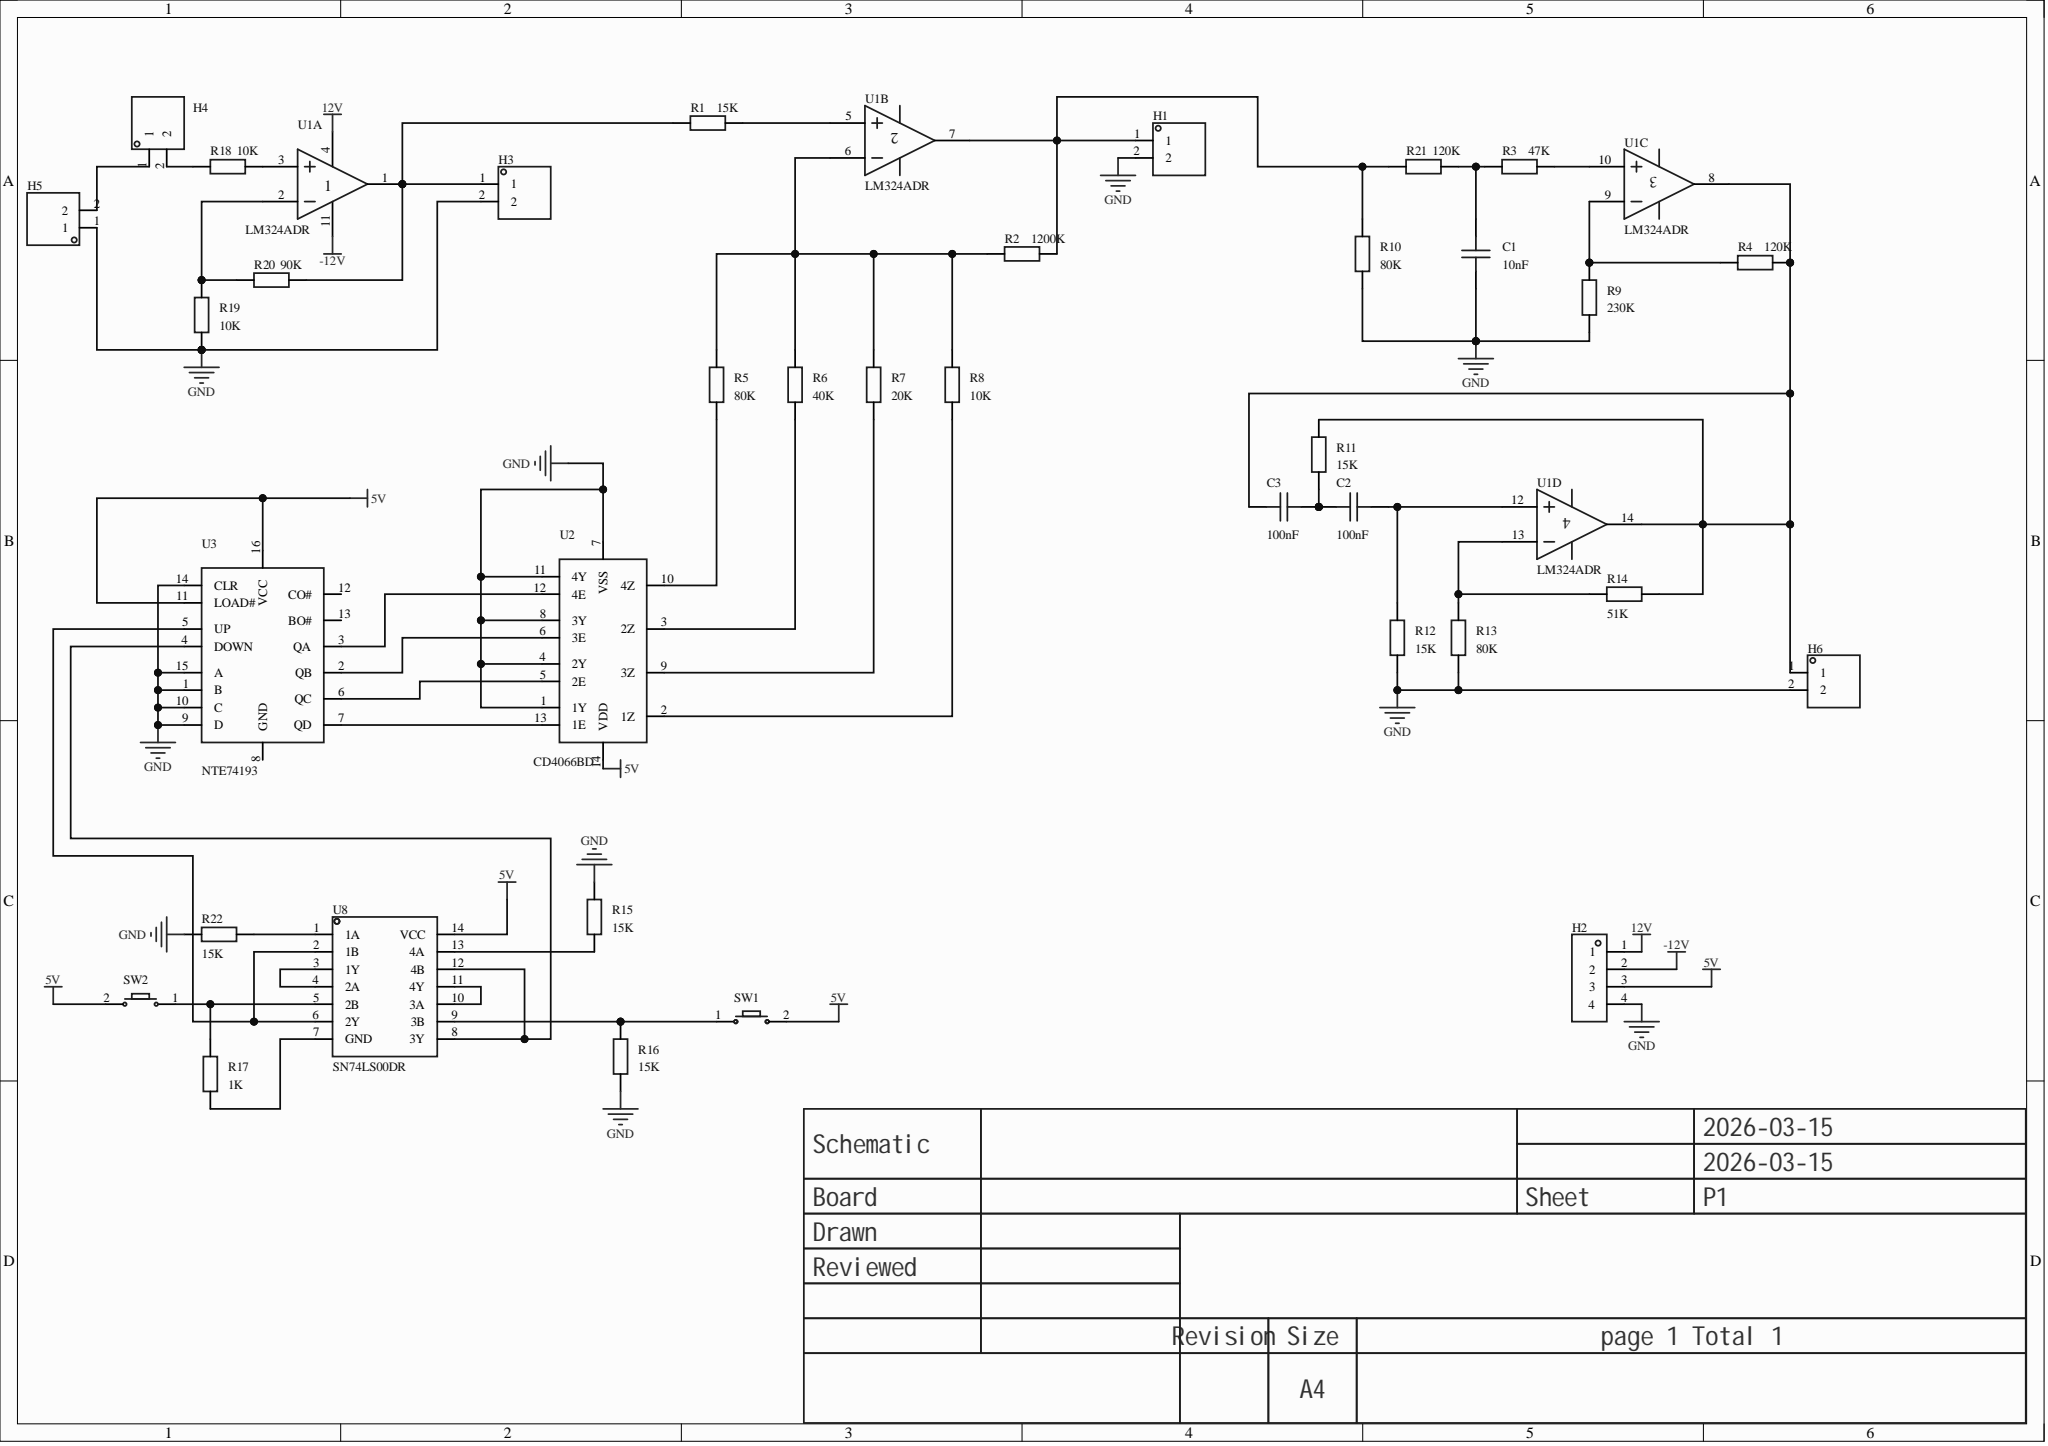Circuit board | Altium Designer | 37 parts | 36 nets
Bill of materials:
Comment,Description,Designator,Footprint,LibRef,Quantity
"10nF","","C1","C0603","CAP_0603","1"
"100nF","","C2, C3","C0603","CAP_0603","2"
"","","H1, H3, H4, H5, H6","HDR-TH_2P-P2.54-V-M-1","HDR-M_2.54_1x2P","5"
"","","H2","HDR-TH_4P-P2.54-V-M","HDR-M_2.54_1x4P","1"
"15K","","R1, R11, R12, R15, R16, R22","R0603","Res_0603","6"
"1200K","","R2","R0603","Res_0603","1"
"47K","","R3","R0603","Res_0603","1"
"120K","","R4, R21","R0603","Res_0603","2"
"80K","","R5, R10, R13","R0603","Res_0603","3"
"40K","","R6","R0603","Res_0603","1"
"20K","","R7","R0603","Res_0603","1"
"10K","","R8, R18, R19","R0603","Res_0603","3"
"230K","","R9","R0603","Res_0603","1"
"51K","","R14","R0603","Res_0603","1"
"1K","","R17","R0603","Res_0603","1"
"90K","","R20","R0603","Res_0603","1"
"","","SW1, SW2","Key_SMD_3x4x2","Key_SMD_3x4x2","2"
"LM324ADR","Amplifiers: four; Rail-to-rail: -; Gain bandwidth product (GBP): -; Input offset voltage (Vos): 9mV; Input bias current (Ib): 250nA;","U1","SOP-14_L8.6-W3.9-P1.27-LS6.0-BL","LM324ADR_C2837469","1"
"CD4066BD","Switch circuit: -; On-resistance (Ron): 1.05kO;","U2","SOP-14_L8.6-W3.9-P1.27-LS6.0-BL","CD4066BD","1"
"NTE74193","Operating voltage: -; Number of elements: 1; Count rate: 32MHz;","U3","PDIP-16_L19.7-W6.6-P2.54-LS7.6-BL","NTE74193","1"
"SN74LS00DR","Logic type: NAND gate; Channels: 4; Operating voltage: 4.75V~5.25V; Propagation delay (tpd): 15ns@5V,15pF;","U8","SOIC-14_L8.7-W3.9-P1.27-LS6.0-BL","SN74LS00DR","1"
Netlist (Protel format):
[
C1
C0603
10nF



]
[
C2
C0603
100nF



]
[
C3
C0603
100nF



]
[
H1
HDR-TH_2P-P2.54-V-M-1




]
[
H2
HDR-TH_4P-P2.54-V-M




]
[
H3
HDR-TH_2P-P2.54-V-M-1




]
[
H4
HDR-TH_2P-P2.54-V-M-1




]
[
H5
HDR-TH_2P-P2.54-V-M-1




]
[
H6
HDR-TH_2P-P2.54-V-M-1




]
[
R1
R0603
15K



]
[
R2
R0603
1200K



]
[
R3
R0603
47K



]
[
R4
R0603
120K



]
[
R5
R0603
80K



]
[
R6
R0603
40K



]
[
R7
R0603
20K



]
[
R8
R0603
10K



]
[
R9
R0603
230K



]
[
R10
R0603
80K



]
[
R11
R0603
15K



]
[
R12
R0603
15K



]
[
R13
R0603
80K



]
[
R14
R0603
51K



]
[
R15
R0603
15K



]
[
R16
R0603
15K



]
[
R17
R0603
1K



]
[
R18
R0603
10K



]
[
R19
R0603
10K



]
[
R20
R0603
90K



]
[
R21
R0603
120K



]
[
R22
R0603
15K



]
[
SW1
Key_SMD_3x4x2




]
[
SW2
Key_SMD_3x4x2




]
[
U1
SOP-14_L8.6-W3.9-P1.27-LS6.0-BL
LM324ADR



]
[
U2
SOP-14_L8.6-W3.9-P1.27-LS6.0-BL
CD4066BD



]
[
U3
PDIP-16_L19.7-W6.6-P2.54-LS7.6-BL
NTE74193



]
[
U8
SOIC-14_L8.7-W3.9-P1.27-LS6.0-BL
SN74LS00DR



]
(
NetU8_10
U8-10
U8-11
)
(
NetU8_3
U8-3
U8-4
)
(
NetU3_5
U3-5
U8-2
U8-6
)
(
NetU3_4
U3-4
U8-8
U8-12
)
(
NetU2_13
U2-13
U3-7
)
(
NetU2_12
U2-12
U3-3
)
(
NetU2_6
U2-6
U3-2
)
(
NetU2_5
U2-5
U3-6
)
(
NetR22_1
R22-1
U8-1
)
(
NetR19_2
R19-2
R20-1
U1-2
)
(
NetR18_2
R18-2
U1-3
)
(
NetR17_2
R17-2
SW2-1
U8-5
)
(
NetR17_1
R17-1
U8-7
)
(
NetR16_2
R16-2
SW1-1
U8-9
)
(
NetR15_1
R15-1
U8-13
)
(
NetR13_2
R13-2
R14-2
U1-13
)
(
NetR8_1
R8-1
U2-2
)
(
NetR7_1
R7-1
U2-9
)
(
NetR6_1
R6-1
U2-3
)
(
NetR5_1
R5-1
U2-10
)
(
NetR4_1
R4-1
R9-2
U1-9
)
(
NetR3_2
R3-2
U1-10
)
(
NetR2_1
R2-1
R5-2
R6-2
R7-2
R8-2
U1-6
)
(
NetR1_2
R1-2
U1-5
)
(
NetH4_2
H4-2
R18-1
)
(
NetH4_1
H4-1
H5-2
)
(
NetH3_1
H3-1
R1-1
R20-2
U1-1
)
(
NetH1_1
H1-1
R2-2
R10-2
R21-1
U1-7
)
(
NetC3_2
C3-2
H6-1
R4-2
R11-2
R14-1
U1-8
U1-14
)
(
NetC2_2
C2-2
C3-1
R11-1
)
(
NetC2_1
C2-1
R12-2
U1-12
)
(
NetC1_2
C1-2
R3-1
R21-2
)
(
GND
C1-1
H1-2
H2-4
H3-2
H5-1
H6-2
R9-1
R10-1
R12-1
R13-1
R15-2
R16-1
R19-1
R22-2
U2-1
U2-4
U2-7
U2-8
U2-11
U3-1
U3-9
U3-10
U3-14
U3-15
)
(
-12V
H2-2
U1-11
)
(
12V
H2-1
U1-4
)
(
5V
H2-3
SW1-2
SW2-2
U2-14
U3-11
U3-16
U8-14
)